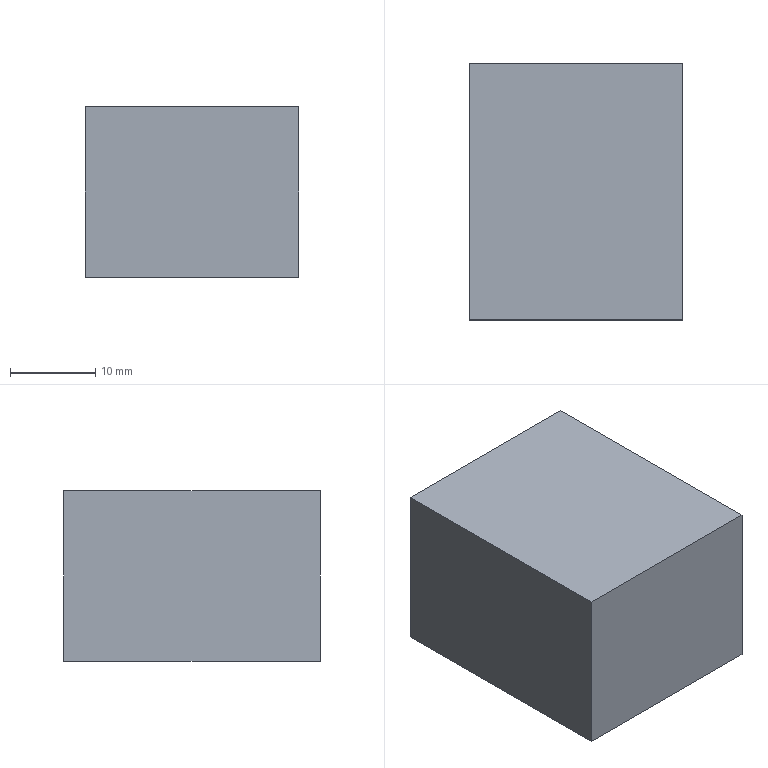Part | STEP file | 20-Positioning block | 1 solid | 6 faces | box 25 x 30 x 20 mm | volume 15000 mm3 | plane 6
STEP:
#1=CARTESIAN_POINT('',(0.,0.,0.));
#2=DIRECTION('',(0.,0.,1.));
#3=DIRECTION('',(1.,0.,0.));
#4=AXIS2_PLACEMENT_3D('',#1,#2,#3);
#5=CARTESIAN_POINT('',(0.,0.,0.));
#6=VERTEX_POINT('',#5);
#7=CARTESIAN_POINT('',(0.,-30.,0.));
#8=VERTEX_POINT('',#7);
#9=CARTESIAN_POINT('',(0.,0.,0.));
#10=DIRECTION('',(0.,-1.,0.));
#11=VECTOR('',#10,1.);
#12=LINE('',#9,#11);
#13=CARTESIAN_POINT('',(0.,0.,20.));
#14=DIRECTION('',(1.,0.,0.));
#15=DIRECTION('',(0.,1.,0.));
#16=AXIS2_PLACEMENT_3D('',#13,#14,#15);
#17=PLANE('',#16);
#18=CARTESIAN_POINT('',(0.,-20.));
#19=DIRECTION('',(-1.,0.));
#20=VECTOR('',#19,1.);
#21=LINE('',#18,#20);
#22=(GEOMETRIC_REPRESENTATION_CONTEXT(2)PARAMETRIC_REPRESENTATION_CONTEXT()REPRESENTATION_CONTEXT('',''));
#23=DEFINITIONAL_REPRESENTATION('',(#21),#22);
#24=PCURVE('',#17,#23);
#25=CARTESIAN_POINT('',(0.,0.,0.));
#26=DIRECTION('',(0.,0.,1.));
#27=DIRECTION('',(1.,0.,0.));
#28=AXIS2_PLACEMENT_3D('',#25,#26,#27);
#29=PLANE('',#28);
#30=CARTESIAN_POINT('',(0.,0.));
#31=DIRECTION('',(0.,-1.));
#32=VECTOR('',#31,1.);
#33=LINE('',#30,#32);
#34=(GEOMETRIC_REPRESENTATION_CONTEXT(2)PARAMETRIC_REPRESENTATION_CONTEXT()REPRESENTATION_CONTEXT('',''));
#35=DEFINITIONAL_REPRESENTATION('',(#33),#34);
#36=PCURVE('',#29,#35);
#37=SURFACE_CURVE('',#12,(#24,#36),.PCURVE_S1.);
#38=EDGE_CURVE('',#6,#8,#37,.T.);
#39=ORIENTED_EDGE('',*,*,#38,.T.);
#40=CARTESIAN_POINT('',(0.,-30.,20.));
#41=VERTEX_POINT('',#40);
#42=CARTESIAN_POINT('',(0.,-30.,20.));
#43=DIRECTION('',(0.,0.,-1.));
#44=VECTOR('',#43,1.);
#45=LINE('',#42,#44);
#46=CARTESIAN_POINT('',(-30.,0.));
#47=DIRECTION('',(0.,-1.));
#48=VECTOR('',#47,1.);
#49=LINE('',#46,#48);
#50=(GEOMETRIC_REPRESENTATION_CONTEXT(2)PARAMETRIC_REPRESENTATION_CONTEXT()REPRESENTATION_CONTEXT('',''));
#51=DEFINITIONAL_REPRESENTATION('',(#49),#50);
#52=PCURVE('',#17,#51);
#53=CARTESIAN_POINT('',(0.,-30.,20.));
#54=DIRECTION('',(0.,1.,0.));
#55=DIRECTION('',(0.,0.,1.));
#56=AXIS2_PLACEMENT_3D('',#53,#54,#55);
#57=PLANE('',#56);
#58=CARTESIAN_POINT('',(0.,0.));
#59=DIRECTION('',(-1.,0.));
#60=VECTOR('',#59,1.);
#61=LINE('',#58,#60);
#62=(GEOMETRIC_REPRESENTATION_CONTEXT(2)PARAMETRIC_REPRESENTATION_CONTEXT()REPRESENTATION_CONTEXT('',''));
#63=DEFINITIONAL_REPRESENTATION('',(#61),#62);
#64=PCURVE('',#57,#63);
#65=SURFACE_CURVE('',#45,(#52,#64),.PCURVE_S1.);
#66=EDGE_CURVE('',#41,#8,#65,.T.);
#67=ORIENTED_EDGE('',*,*,#66,.F.);
#68=CARTESIAN_POINT('',(0.,0.,20.));
#69=VERTEX_POINT('',#68);
#70=CARTESIAN_POINT('',(0.,0.,20.));
#71=DIRECTION('',(0.,-1.,0.));
#72=VECTOR('',#71,1.);
#73=LINE('',#70,#72);
#74=CARTESIAN_POINT('',(0.,0.));
#75=DIRECTION('',(-1.,0.));
#76=VECTOR('',#75,1.);
#77=LINE('',#74,#76);
#78=(GEOMETRIC_REPRESENTATION_CONTEXT(2)PARAMETRIC_REPRESENTATION_CONTEXT()REPRESENTATION_CONTEXT('',''));
#79=DEFINITIONAL_REPRESENTATION('',(#77),#78);
#80=PCURVE('',#17,#79);
#81=CARTESIAN_POINT('',(0.,0.,20.));
#82=DIRECTION('',(0.,0.,1.));
#83=DIRECTION('',(1.,0.,0.));
#84=AXIS2_PLACEMENT_3D('',#81,#82,#83);
#85=PLANE('',#84);
#86=CARTESIAN_POINT('',(0.,0.));
#87=DIRECTION('',(0.,-1.));
#88=VECTOR('',#87,1.);
#89=LINE('',#86,#88);
#90=(GEOMETRIC_REPRESENTATION_CONTEXT(2)PARAMETRIC_REPRESENTATION_CONTEXT()REPRESENTATION_CONTEXT('',''));
#91=DEFINITIONAL_REPRESENTATION('',(#89),#90);
#92=PCURVE('',#85,#91);
#93=SURFACE_CURVE('',#73,(#80,#92),.PCURVE_S1.);
#94=EDGE_CURVE('',#69,#41,#93,.T.);
#95=ORIENTED_EDGE('',*,*,#94,.F.);
#96=CARTESIAN_POINT('',(0.,0.,20.));
#97=DIRECTION('',(0.,0.,-1.));
#98=VECTOR('',#97,1.);
#99=LINE('',#96,#98);
#100=CARTESIAN_POINT('',(0.,0.));
#101=DIRECTION('',(0.,-1.));
#102=VECTOR('',#101,1.);
#103=LINE('',#100,#102);
#104=(GEOMETRIC_REPRESENTATION_CONTEXT(2)PARAMETRIC_REPRESENTATION_CONTEXT()REPRESENTATION_CONTEXT('',''));
#105=DEFINITIONAL_REPRESENTATION('',(#103),#104);
#106=PCURVE('',#17,#105);
#107=CARTESIAN_POINT('',(0.,0.,20.));
#108=DIRECTION('',(0.,-1.,0.));
#109=DIRECTION('',(0.,0.,-1.));
#110=AXIS2_PLACEMENT_3D('',#107,#108,#109);
#111=PLANE('',#110);
#112=CARTESIAN_POINT('',(0.,0.));
#113=DIRECTION('',(1.,0.));
#114=VECTOR('',#113,1.);
#115=LINE('',#112,#114);
#116=(GEOMETRIC_REPRESENTATION_CONTEXT(2)PARAMETRIC_REPRESENTATION_CONTEXT()REPRESENTATION_CONTEXT('',''));
#117=DEFINITIONAL_REPRESENTATION('',(#115),#116);
#118=PCURVE('',#111,#117);
#119=SURFACE_CURVE('',#99,(#106,#118),.PCURVE_S1.);
#120=EDGE_CURVE('',#69,#6,#119,.T.);
#121=ORIENTED_EDGE('',*,*,#120,.T.);
#122=EDGE_LOOP('',(#39,#67,#95,#121));
#123=FACE_BOUND('',#122,.T.);
#124=ADVANCED_FACE('',(#123),#17,.F.);
#125=CARTESIAN_POINT('',(25.,-30.,0.));
#126=VERTEX_POINT('',#125);
#127=CARTESIAN_POINT('',(0.,-30.,0.));
#128=DIRECTION('',(1.,0.,0.));
#129=VECTOR('',#128,1.);
#130=LINE('',#127,#129);
#131=CARTESIAN_POINT('',(-20.,0.));
#132=DIRECTION('',(0.,1.));
#133=VECTOR('',#132,1.);
#134=LINE('',#131,#133);
#135=(GEOMETRIC_REPRESENTATION_CONTEXT(2)PARAMETRIC_REPRESENTATION_CONTEXT()REPRESENTATION_CONTEXT('',''));
#136=DEFINITIONAL_REPRESENTATION('',(#134),#135);
#137=PCURVE('',#57,#136);
#138=CARTESIAN_POINT('',(0.,-30.));
#139=DIRECTION('',(1.,0.));
#140=VECTOR('',#139,1.);
#141=LINE('',#138,#140);
#142=(GEOMETRIC_REPRESENTATION_CONTEXT(2)PARAMETRIC_REPRESENTATION_CONTEXT()REPRESENTATION_CONTEXT('',''));
#143=DEFINITIONAL_REPRESENTATION('',(#141),#142);
#144=PCURVE('',#29,#143);
#145=SURFACE_CURVE('',#130,(#137,#144),.PCURVE_S1.);
#146=EDGE_CURVE('',#8,#126,#145,.T.);
#147=ORIENTED_EDGE('',*,*,#146,.T.);
#148=CARTESIAN_POINT('',(25.,-30.,20.));
#149=VERTEX_POINT('',#148);
#150=CARTESIAN_POINT('',(25.,-30.,20.));
#151=DIRECTION('',(0.,0.,-1.));
#152=VECTOR('',#151,1.);
#153=LINE('',#150,#152);
#154=CARTESIAN_POINT('',(0.,25.));
#155=DIRECTION('',(-1.,0.));
#156=VECTOR('',#155,1.);
#157=LINE('',#154,#156);
#158=(GEOMETRIC_REPRESENTATION_CONTEXT(2)PARAMETRIC_REPRESENTATION_CONTEXT()REPRESENTATION_CONTEXT('',''));
#159=DEFINITIONAL_REPRESENTATION('',(#157),#158);
#160=PCURVE('',#57,#159);
#161=CARTESIAN_POINT('',(25.,0.,20.));
#162=DIRECTION('',(-1.,0.,0.));
#163=DIRECTION('',(0.,-1.,0.));
#164=AXIS2_PLACEMENT_3D('',#161,#162,#163);
#165=PLANE('',#164);
#166=CARTESIAN_POINT('',(30.,0.));
#167=DIRECTION('',(0.,-1.));
#168=VECTOR('',#167,1.);
#169=LINE('',#166,#168);
#170=(GEOMETRIC_REPRESENTATION_CONTEXT(2)PARAMETRIC_REPRESENTATION_CONTEXT()REPRESENTATION_CONTEXT('',''));
#171=DEFINITIONAL_REPRESENTATION('',(#169),#170);
#172=PCURVE('',#165,#171);
#173=SURFACE_CURVE('',#153,(#160,#172),.PCURVE_S1.);
#174=EDGE_CURVE('',#149,#126,#173,.T.);
#175=ORIENTED_EDGE('',*,*,#174,.F.);
#176=CARTESIAN_POINT('',(0.,-30.,20.));
#177=DIRECTION('',(1.,0.,0.));
#178=VECTOR('',#177,1.);
#179=LINE('',#176,#178);
#180=CARTESIAN_POINT('',(0.,0.));
#181=DIRECTION('',(0.,1.));
#182=VECTOR('',#181,1.);
#183=LINE('',#180,#182);
#184=(GEOMETRIC_REPRESENTATION_CONTEXT(2)PARAMETRIC_REPRESENTATION_CONTEXT()REPRESENTATION_CONTEXT('',''));
#185=DEFINITIONAL_REPRESENTATION('',(#183),#184);
#186=PCURVE('',#57,#185);
#187=CARTESIAN_POINT('',(0.,-30.));
#188=DIRECTION('',(1.,0.));
#189=VECTOR('',#188,1.);
#190=LINE('',#187,#189);
#191=(GEOMETRIC_REPRESENTATION_CONTEXT(2)PARAMETRIC_REPRESENTATION_CONTEXT()REPRESENTATION_CONTEXT('',''));
#192=DEFINITIONAL_REPRESENTATION('',(#190),#191);
#193=PCURVE('',#85,#192);
#194=SURFACE_CURVE('',#179,(#186,#193),.PCURVE_S1.);
#195=EDGE_CURVE('',#41,#149,#194,.T.);
#196=ORIENTED_EDGE('',*,*,#195,.F.);
#197=ORIENTED_EDGE('',*,*,#66,.T.);
#198=EDGE_LOOP('',(#147,#175,#196,#197));
#199=FACE_BOUND('',#198,.T.);
#200=ADVANCED_FACE('',(#199),#57,.F.);
#201=CARTESIAN_POINT('',(25.,0.,0.));
#202=VERTEX_POINT('',#201);
#203=CARTESIAN_POINT('',(25.,0.,0.));
#204=DIRECTION('',(0.,1.,0.));
#205=VECTOR('',#204,1.);
#206=LINE('',#203,#205);
#207=CARTESIAN_POINT('',(0.,-20.));
#208=DIRECTION('',(-1.,0.));
#209=VECTOR('',#208,1.);
#210=LINE('',#207,#209);
#211=(GEOMETRIC_REPRESENTATION_CONTEXT(2)PARAMETRIC_REPRESENTATION_CONTEXT()REPRESENTATION_CONTEXT('',''));
#212=DEFINITIONAL_REPRESENTATION('',(#210),#211);
#213=PCURVE('',#165,#212);
#214=CARTESIAN_POINT('',(25.,0.));
#215=DIRECTION('',(0.,1.));
#216=VECTOR('',#215,1.);
#217=LINE('',#214,#216);
#218=(GEOMETRIC_REPRESENTATION_CONTEXT(2)PARAMETRIC_REPRESENTATION_CONTEXT()REPRESENTATION_CONTEXT('',''));
#219=DEFINITIONAL_REPRESENTATION('',(#217),#218);
#220=PCURVE('',#29,#219);
#221=SURFACE_CURVE('',#206,(#213,#220),.PCURVE_S1.);
#222=EDGE_CURVE('',#126,#202,#221,.T.);
#223=ORIENTED_EDGE('',*,*,#222,.T.);
#224=CARTESIAN_POINT('',(25.,0.,20.));
#225=VERTEX_POINT('',#224);
#226=CARTESIAN_POINT('',(25.,0.,20.));
#227=DIRECTION('',(0.,0.,-1.));
#228=VECTOR('',#227,1.);
#229=LINE('',#226,#228);
#230=CARTESIAN_POINT('',(0.,0.));
#231=DIRECTION('',(0.,-1.));
#232=VECTOR('',#231,1.);
#233=LINE('',#230,#232);
#234=(GEOMETRIC_REPRESENTATION_CONTEXT(2)PARAMETRIC_REPRESENTATION_CONTEXT()REPRESENTATION_CONTEXT('',''));
#235=DEFINITIONAL_REPRESENTATION('',(#233),#234);
#236=PCURVE('',#165,#235);
#237=CARTESIAN_POINT('',(0.,25.));
#238=DIRECTION('',(1.,0.));
#239=VECTOR('',#238,1.);
#240=LINE('',#237,#239);
#241=(GEOMETRIC_REPRESENTATION_CONTEXT(2)PARAMETRIC_REPRESENTATION_CONTEXT()REPRESENTATION_CONTEXT('',''));
#242=DEFINITIONAL_REPRESENTATION('',(#240),#241);
#243=PCURVE('',#111,#242);
#244=SURFACE_CURVE('',#229,(#236,#243),.PCURVE_S1.);
#245=EDGE_CURVE('',#225,#202,#244,.T.);
#246=ORIENTED_EDGE('',*,*,#245,.F.);
#247=CARTESIAN_POINT('',(25.,0.,20.));
#248=DIRECTION('',(0.,1.,0.));
#249=VECTOR('',#248,1.);
#250=LINE('',#247,#249);
#251=CARTESIAN_POINT('',(0.,0.));
#252=DIRECTION('',(-1.,0.));
#253=VECTOR('',#252,1.);
#254=LINE('',#251,#253);
#255=(GEOMETRIC_REPRESENTATION_CONTEXT(2)PARAMETRIC_REPRESENTATION_CONTEXT()REPRESENTATION_CONTEXT('',''));
#256=DEFINITIONAL_REPRESENTATION('',(#254),#255);
#257=PCURVE('',#165,#256);
#258=CARTESIAN_POINT('',(25.,0.));
#259=DIRECTION('',(0.,1.));
#260=VECTOR('',#259,1.);
#261=LINE('',#258,#260);
#262=(GEOMETRIC_REPRESENTATION_CONTEXT(2)PARAMETRIC_REPRESENTATION_CONTEXT()REPRESENTATION_CONTEXT('',''));
#263=DEFINITIONAL_REPRESENTATION('',(#261),#262);
#264=PCURVE('',#85,#263);
#265=SURFACE_CURVE('',#250,(#257,#264),.PCURVE_S1.);
#266=EDGE_CURVE('',#149,#225,#265,.T.);
#267=ORIENTED_EDGE('',*,*,#266,.F.);
#268=ORIENTED_EDGE('',*,*,#174,.T.);
#269=EDGE_LOOP('',(#223,#246,#267,#268));
#270=FACE_BOUND('',#269,.T.);
#271=ADVANCED_FACE('',(#270),#165,.F.);
#272=CARTESIAN_POINT('',(0.,0.,0.));
#273=DIRECTION('',(-1.,0.,0.));
#274=VECTOR('',#273,1.);
#275=LINE('',#272,#274);
#276=CARTESIAN_POINT('',(20.,0.));
#277=DIRECTION('',(0.,-1.));
#278=VECTOR('',#277,1.);
#279=LINE('',#276,#278);
#280=(GEOMETRIC_REPRESENTATION_CONTEXT(2)PARAMETRIC_REPRESENTATION_CONTEXT()REPRESENTATION_CONTEXT('',''));
#281=DEFINITIONAL_REPRESENTATION('',(#279),#280);
#282=PCURVE('',#111,#281);
#283=CARTESIAN_POINT('',(0.,0.));
#284=DIRECTION('',(-1.,0.));
#285=VECTOR('',#284,1.);
#286=LINE('',#283,#285);
#287=(GEOMETRIC_REPRESENTATION_CONTEXT(2)PARAMETRIC_REPRESENTATION_CONTEXT()REPRESENTATION_CONTEXT('',''));
#288=DEFINITIONAL_REPRESENTATION('',(#286),#287);
#289=PCURVE('',#29,#288);
#290=SURFACE_CURVE('',#275,(#282,#289),.PCURVE_S1.);
#291=EDGE_CURVE('',#202,#6,#290,.T.);
#292=ORIENTED_EDGE('',*,*,#291,.T.);
#293=ORIENTED_EDGE('',*,*,#120,.F.);
#294=CARTESIAN_POINT('',(0.,0.,20.));
#295=DIRECTION('',(-1.,0.,0.));
#296=VECTOR('',#295,1.);
#297=LINE('',#294,#296);
#298=CARTESIAN_POINT('',(0.,0.));
#299=DIRECTION('',(0.,-1.));
#300=VECTOR('',#299,1.);
#301=LINE('',#298,#300);
#302=(GEOMETRIC_REPRESENTATION_CONTEXT(2)PARAMETRIC_REPRESENTATION_CONTEXT()REPRESENTATION_CONTEXT('',''));
#303=DEFINITIONAL_REPRESENTATION('',(#301),#302);
#304=PCURVE('',#111,#303);
#305=CARTESIAN_POINT('',(0.,0.));
#306=DIRECTION('',(-1.,0.));
#307=VECTOR('',#306,1.);
#308=LINE('',#305,#307);
#309=(GEOMETRIC_REPRESENTATION_CONTEXT(2)PARAMETRIC_REPRESENTATION_CONTEXT()REPRESENTATION_CONTEXT('',''));
#310=DEFINITIONAL_REPRESENTATION('',(#308),#309);
#311=PCURVE('',#85,#310);
#312=SURFACE_CURVE('',#297,(#304,#311),.PCURVE_S1.);
#313=EDGE_CURVE('',#225,#69,#312,.T.);
#314=ORIENTED_EDGE('',*,*,#313,.F.);
#315=ORIENTED_EDGE('',*,*,#245,.T.);
#316=EDGE_LOOP('',(#292,#293,#314,#315));
#317=FACE_BOUND('',#316,.T.);
#318=ADVANCED_FACE('',(#317),#111,.F.);
#319=ORIENTED_EDGE('',*,*,#94,.T.);
#320=ORIENTED_EDGE('',*,*,#195,.T.);
#321=ORIENTED_EDGE('',*,*,#266,.T.);
#322=ORIENTED_EDGE('',*,*,#313,.T.);
#323=EDGE_LOOP('',(#319,#320,#321,#322));
#324=FACE_BOUND('',#323,.T.);
#325=ADVANCED_FACE('',(#324),#85,.T.);
#326=ORIENTED_EDGE('',*,*,#38,.F.);
#327=ORIENTED_EDGE('',*,*,#291,.F.);
#328=ORIENTED_EDGE('',*,*,#222,.F.);
#329=ORIENTED_EDGE('',*,*,#146,.F.);
#330=EDGE_LOOP('',(#326,#327,#328,#329));
#331=FACE_BOUND('',#330,.T.);
#332=ADVANCED_FACE('',(#331),#29,.F.);
#333=CLOSED_SHELL('',(#124,#200,#271,#318,#325,#332));
#334=MANIFOLD_SOLID_BREP('',#333);
#335=(LENGTH_UNIT()NAMED_UNIT(*)SI_UNIT(.MILLI.,.METRE.));
#336=UNCERTAINTY_MEASURE_WITH_UNIT(LENGTH_MEASURE(0.0000001),#335,'','');
#337=(NAMED_UNIT(*)PLANE_ANGLE_UNIT()SI_UNIT($,.RADIAN.));
#338=(NAMED_UNIT(*)SI_UNIT($,.STERADIAN.)SOLID_ANGLE_UNIT());
#339=(GEOMETRIC_REPRESENTATION_CONTEXT(3)GLOBAL_UNCERTAINTY_ASSIGNED_CONTEXT((#336))GLOBAL_UNIT_ASSIGNED_CONTEXT((#335,#337,#338))REPRESENTATION_CONTEXT('',''));
#340=ADVANCED_BREP_SHAPE_REPRESENTATION('',(#4,#334),#339);